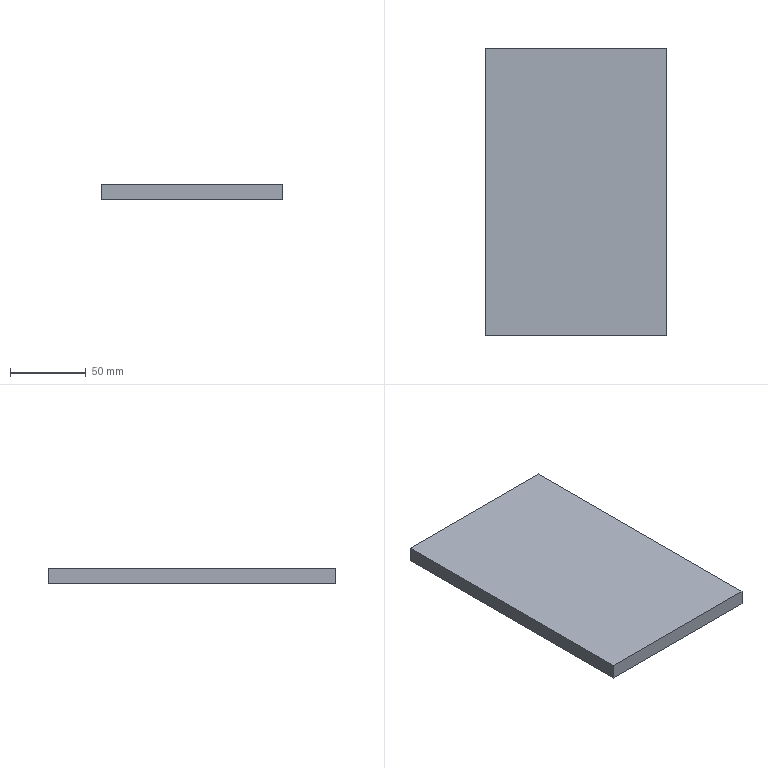Part | STEP file | MYT-A01-P42 | 1 solid | 6 faces | box 120 x 190 x 10 mm | volume 228000 mm3 | plane 6
STEP:
#1=CARTESIAN_POINT('',(60.,-95.,0.));
#2=VERTEX_POINT('',#1);
#3=CARTESIAN_POINT('',(60.,95.,0.));
#4=VERTEX_POINT('',#3);
#5=CARTESIAN_POINT('',(60.,95.,0.));
#6=DIRECTION('',(0.,1.,0.));
#7=VECTOR('',#6,1000.);
#8=LINE('',#5,#7);
#9=EDGE_CURVE('',#2,#4,#8,.T.);
#10=ORIENTED_EDGE('',*,*,#9,.T.);
#11=CARTESIAN_POINT('',(60.,95.,10.));
#12=VERTEX_POINT('',#11);
#13=CARTESIAN_POINT('',(60.,95.,10.));
#14=DIRECTION('',(0.,0.,-1.));
#15=VECTOR('',#14,1000.);
#16=LINE('',#13,#15);
#17=EDGE_CURVE('',#12,#4,#16,.T.);
#18=ORIENTED_EDGE('',*,*,#17,.F.);
#19=CARTESIAN_POINT('',(60.,-95.,10.));
#20=VERTEX_POINT('',#19);
#21=CARTESIAN_POINT('',(60.,95.,10.));
#22=DIRECTION('',(0.,1.,0.));
#23=VECTOR('',#22,1000.);
#24=LINE('',#21,#23);
#25=EDGE_CURVE('',#20,#12,#24,.T.);
#26=ORIENTED_EDGE('',*,*,#25,.F.);
#27=CARTESIAN_POINT('',(60.,-95.,10.));
#28=DIRECTION('',(0.,0.,-1.));
#29=VECTOR('',#28,1000.);
#30=LINE('',#27,#29);
#31=EDGE_CURVE('',#20,#2,#30,.T.);
#32=ORIENTED_EDGE('',*,*,#31,.T.);
#33=EDGE_LOOP('',(#10,#18,#26,#32));
#34=FACE_OUTER_BOUND('',#33,.T.);
#35=CARTESIAN_POINT('',(60.,95.,10.));
#36=DIRECTION('',(-1.,0.,0.));
#37=DIRECTION('',(0.,-1.,0.));
#38=AXIS2_PLACEMENT_3D('',#35,#36,#37);
#39=PLANE('',#38);
#40=ADVANCED_FACE('',(#34),#39,.F.);
#41=CARTESIAN_POINT('',(-60.,95.,0.));
#42=VERTEX_POINT('',#41);
#43=CARTESIAN_POINT('',(-60.,95.,0.));
#44=DIRECTION('',(-1.,0.,0.));
#45=VECTOR('',#44,1000.);
#46=LINE('',#43,#45);
#47=EDGE_CURVE('',#4,#42,#46,.T.);
#48=ORIENTED_EDGE('',*,*,#47,.T.);
#49=CARTESIAN_POINT('',(-60.,95.,10.));
#50=VERTEX_POINT('',#49);
#51=CARTESIAN_POINT('',(-60.,95.,10.));
#52=DIRECTION('',(0.,0.,-1.));
#53=VECTOR('',#52,1000.);
#54=LINE('',#51,#53);
#55=EDGE_CURVE('',#50,#42,#54,.T.);
#56=ORIENTED_EDGE('',*,*,#55,.F.);
#57=CARTESIAN_POINT('',(-60.,95.,10.));
#58=DIRECTION('',(-1.,0.,0.));
#59=VECTOR('',#58,1000.);
#60=LINE('',#57,#59);
#61=EDGE_CURVE('',#12,#50,#60,.T.);
#62=ORIENTED_EDGE('',*,*,#61,.F.);
#63=ORIENTED_EDGE('',*,*,#17,.T.);
#64=EDGE_LOOP('',(#48,#56,#62,#63));
#65=FACE_OUTER_BOUND('',#64,.T.);
#66=CARTESIAN_POINT('',(-60.,95.,10.));
#67=DIRECTION('',(0.,-1.,0.));
#68=DIRECTION('',(0.,0.,-1.));
#69=AXIS2_PLACEMENT_3D('',#66,#67,#68);
#70=PLANE('',#69);
#71=ADVANCED_FACE('',(#65),#70,.F.);
#72=CARTESIAN_POINT('',(-60.,-95.,0.));
#73=VERTEX_POINT('',#72);
#74=CARTESIAN_POINT('',(-60.,95.,0.));
#75=DIRECTION('',(0.,-1.,0.));
#76=VECTOR('',#75,1000.);
#77=LINE('',#74,#76);
#78=EDGE_CURVE('',#42,#73,#77,.T.);
#79=ORIENTED_EDGE('',*,*,#78,.T.);
#80=CARTESIAN_POINT('',(-60.,-95.,10.));
#81=VERTEX_POINT('',#80);
#82=CARTESIAN_POINT('',(-60.,-95.,10.));
#83=DIRECTION('',(0.,0.,-1.));
#84=VECTOR('',#83,1000.);
#85=LINE('',#82,#84);
#86=EDGE_CURVE('',#81,#73,#85,.T.);
#87=ORIENTED_EDGE('',*,*,#86,.F.);
#88=CARTESIAN_POINT('',(-60.,95.,10.));
#89=DIRECTION('',(0.,-1.,0.));
#90=VECTOR('',#89,1000.);
#91=LINE('',#88,#90);
#92=EDGE_CURVE('',#50,#81,#91,.T.);
#93=ORIENTED_EDGE('',*,*,#92,.F.);
#94=ORIENTED_EDGE('',*,*,#55,.T.);
#95=EDGE_LOOP('',(#79,#87,#93,#94));
#96=FACE_OUTER_BOUND('',#95,.T.);
#97=CARTESIAN_POINT('',(-60.,95.,10.));
#98=DIRECTION('',(1.,0.,0.));
#99=DIRECTION('',(0.,1.,0.));
#100=AXIS2_PLACEMENT_3D('',#97,#98,#99);
#101=PLANE('',#100);
#102=ADVANCED_FACE('',(#96),#101,.F.);
#103=CARTESIAN_POINT('',(-60.,-95.,0.));
#104=DIRECTION('',(1.,0.,0.));
#105=VECTOR('',#104,1000.);
#106=LINE('',#103,#105);
#107=EDGE_CURVE('',#73,#2,#106,.T.);
#108=ORIENTED_EDGE('',*,*,#107,.T.);
#109=ORIENTED_EDGE('',*,*,#31,.F.);
#110=CARTESIAN_POINT('',(-60.,-95.,10.));
#111=DIRECTION('',(1.,0.,0.));
#112=VECTOR('',#111,1000.);
#113=LINE('',#110,#112);
#114=EDGE_CURVE('',#81,#20,#113,.T.);
#115=ORIENTED_EDGE('',*,*,#114,.F.);
#116=ORIENTED_EDGE('',*,*,#86,.T.);
#117=EDGE_LOOP('',(#108,#109,#115,#116));
#118=FACE_OUTER_BOUND('',#117,.T.);
#119=CARTESIAN_POINT('',(-60.,-95.,10.));
#120=DIRECTION('',(0.,1.,0.));
#121=DIRECTION('',(0.,0.,1.));
#122=AXIS2_PLACEMENT_3D('',#119,#120,#121);
#123=PLANE('',#122);
#124=ADVANCED_FACE('',(#118),#123,.F.);
#125=ORIENTED_EDGE('',*,*,#25,.T.);
#126=ORIENTED_EDGE('',*,*,#61,.T.);
#127=ORIENTED_EDGE('',*,*,#92,.T.);
#128=ORIENTED_EDGE('',*,*,#114,.T.);
#129=EDGE_LOOP('',(#125,#126,#127,#128));
#130=FACE_OUTER_BOUND('',#129,.T.);
#131=CARTESIAN_POINT('',(0.,0.,10.));
#132=DIRECTION('',(0.,0.,1.));
#133=DIRECTION('',(1.,0.,0.));
#134=AXIS2_PLACEMENT_3D('',#131,#132,#133);
#135=PLANE('',#134);
#136=ADVANCED_FACE('',(#130),#135,.T.);
#137=ORIENTED_EDGE('',*,*,#9,.F.);
#138=ORIENTED_EDGE('',*,*,#107,.F.);
#139=ORIENTED_EDGE('',*,*,#78,.F.);
#140=ORIENTED_EDGE('',*,*,#47,.F.);
#141=EDGE_LOOP('',(#137,#138,#139,#140));
#142=FACE_OUTER_BOUND('',#141,.T.);
#143=CARTESIAN_POINT('',(0.,0.,0.));
#144=DIRECTION('',(0.,0.,1.));
#145=DIRECTION('',(1.,0.,0.));
#146=AXIS2_PLACEMENT_3D('',#143,#144,#145);
#147=PLANE('',#146);
#148=ADVANCED_FACE('',(#142),#147,.F.);
#149=CLOSED_SHELL('',(#40,#71,#102,#124,#136,#148));
#150=MANIFOLD_SOLID_BREP('',#149);
#151=CARTESIAN_POINT('',(0.,0.,0.));
#152=DIRECTION('',(0.,0.,1.));
#153=DIRECTION('',(1.,0.,0.));
#154=AXIS2_PLACEMENT_3D('',#151,#152,#153);
#155=(LENGTH_UNIT()NAMED_UNIT(*)SI_UNIT(.MILLI.,.METRE.));
#156=UNCERTAINTY_MEASURE_WITH_UNIT(LENGTH_MEASURE(0.00001),#155,'','');
#157=(NAMED_UNIT(*)PLANE_ANGLE_UNIT()SI_UNIT($,.RADIAN.));
#158=(NAMED_UNIT(*)SI_UNIT($,.STERADIAN.)SOLID_ANGLE_UNIT());
#159=(GEOMETRIC_REPRESENTATION_CONTEXT(3)GLOBAL_UNCERTAINTY_ASSIGNED_CONTEXT((#156))GLOBAL_UNIT_ASSIGNED_CONTEXT((#155,#157,#158))REPRESENTATION_CONTEXT('',''));
#160=ADVANCED_BREP_SHAPE_REPRESENTATION('',(#150,#154),#159);